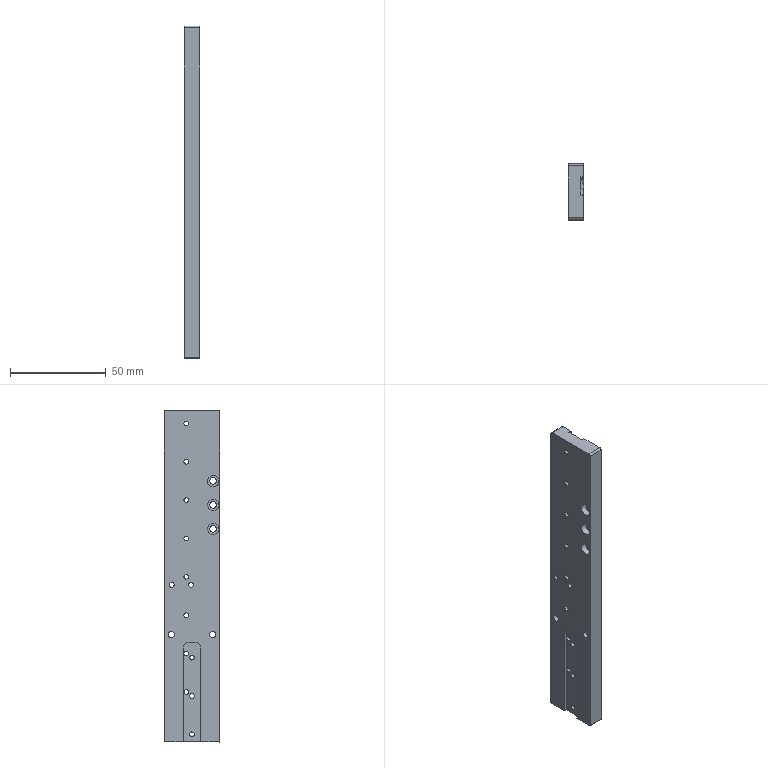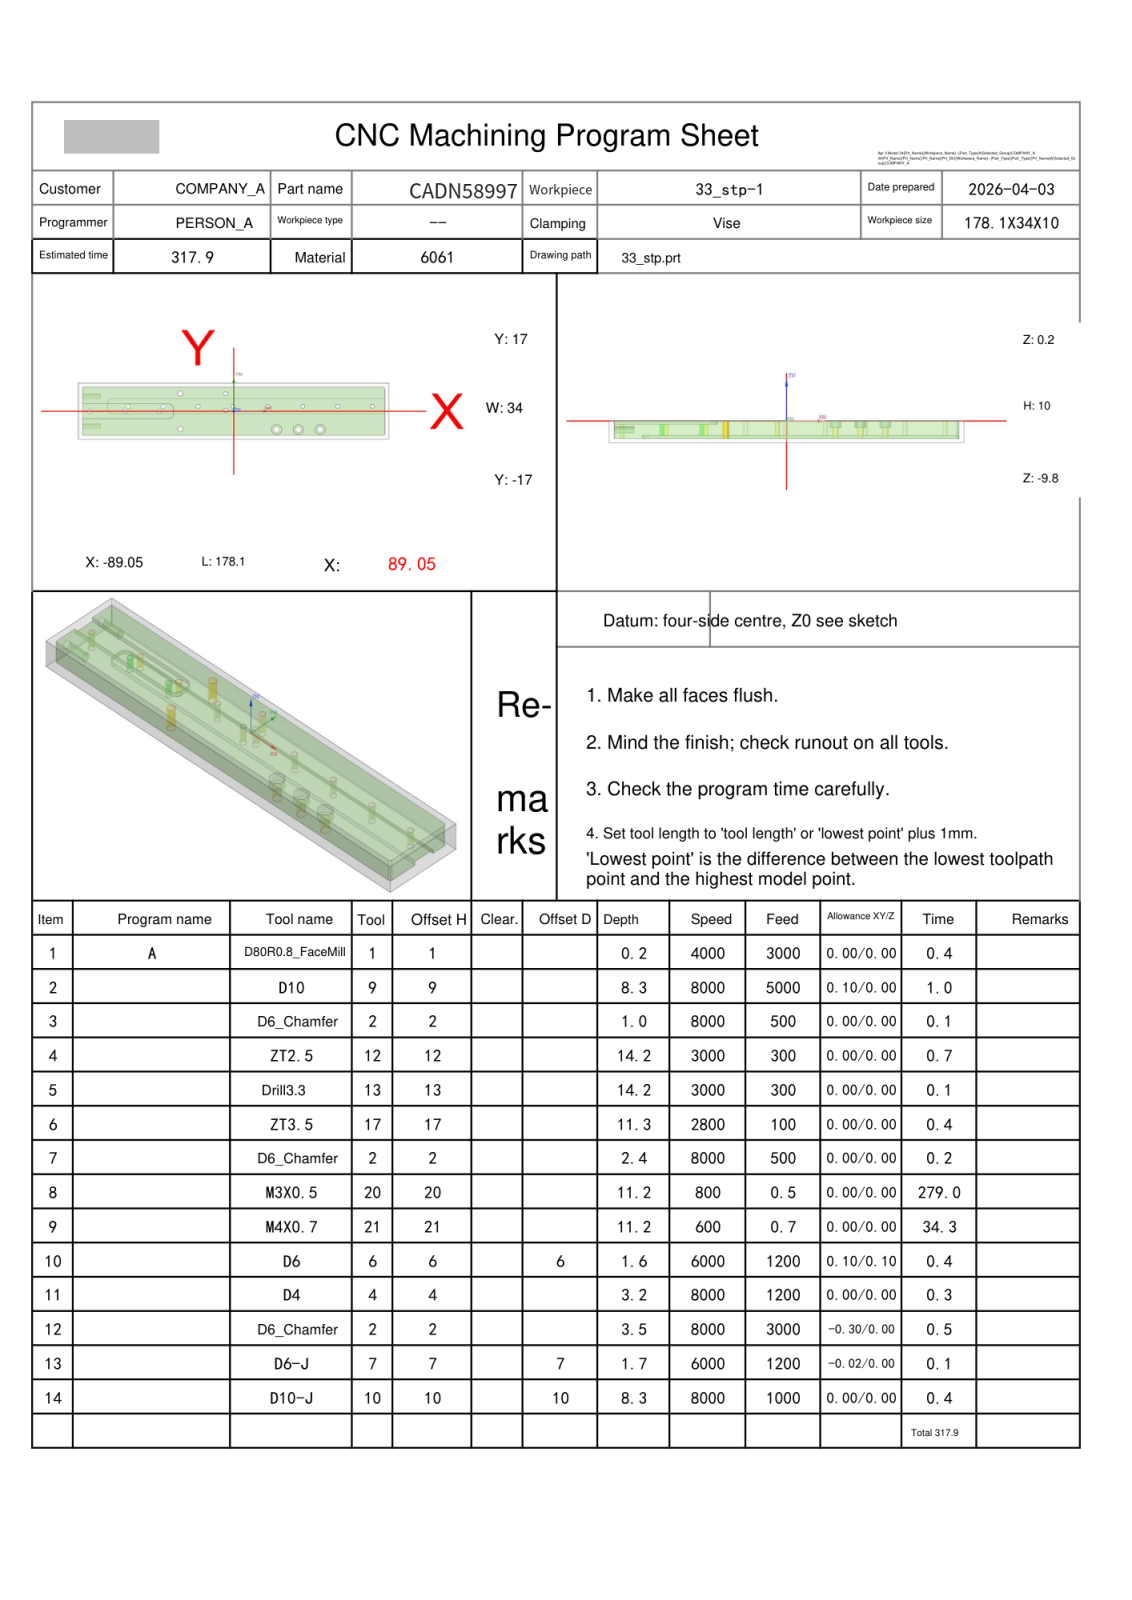NC program | NX | posted by the shop | part box 8 x 29 x 173.1 mm
Whole program:
%
O0001
(Machine time: 605.15 MIN)
(===Total Tool:12===)
(T1=D80R0.8 FaceMill D=80.  R=0.8  D-  H01 Z=-0.   )
(T9=D10     D=10.  R=0.   D-  H09 Z=-8.1  )
(T2=D6 Chamfer   D=6.   R=0.   D-  H02 Z=-3.25 )
(T12=ZT2.5  D=2.5  DR_a=118 D-  H12 Z=-14.  )
(T13=Drill 3.3  D=3.3  DR_a=118 D-  H13 Z=-13.99)
(T17=ZT3.5  D=3.5  DR_a=118 D-  H17 Z=-11.05)
(T20=M3X0.5 D=2.5  DR_a=180 D-  H20 Z=-11.  )
(T21=M4X0.7 D=3.3  DR_a=180 D-  H21 Z=-11.  )
(T6=D6      D=6.   R=0.   D6  H06 Z=-1.4  )
(T4=D4      D=4.   R=0.   D4  H04 Z=-3.   )
(T7=D6-J    D=6.   R=0.   D7  H07 Z=-1.5  )
(T10=D10-J  D=10.  R=0.   D10 H10 Z=-8.1  )
G80 G90 G17 G49 G40
G91 G28 Z0
M01
N1 T01 M06
(D80R0.8 FaceMill  D=80. R=0.8 H=01 ce=0.20 di=0.10)
G00 G90 G54 X-131.55 Y0.0 M03 S4000
G43 H01 Z20.
M08
Z2.1
G01 Z.1 F3000.
X-126.55
X126.55
X131.55
Z2.1
G00 Z20.
G00 G90 X-131.55 Y0.0 M03 S4000
Z20.
Z2.
G01 Z0.0 F1000.
X-126.55
X126.55
X131.55
Z2.
G00 Z20.
G91 G28 Z0.0
M05
M09
G91 G28 Z0.0
M01
N2 T09 M06
(D10  D=10. R=0. H=09 ce=0.10 di=0.00)
G00 G90 G54 X-.4 Y-19.6 M03 S8000
G43 H09 Z20.
M08
Z.5
G01 X-86.35 Z.346 F5000.
G02 X-89.956 Y-18.106 Z.338 I0.0 J5.1
G01 X-90.156 Y-17.906
G02 X-91.65 Y-14.3 Z.331 I3.606 J3.606
G01 Y14.3 Z.279
G02 X-90.156 Y17.906 Z.272 I5.1 J0.0
G01 X-89.956 Y18.106
G02 X-86.35 Y19.6 Z.264 I3.606 J-3.606
G01 X85.55 Z-.044
G02 X91.65 Y13.5 Z-.062 I0.0 J-6.1
G01 Y-13.5 Z-.11
G02 X89.12 Y-18.446 Z-.121 I-6.1 J0.0
X85.55 Y-19.6 Z-.127 I-3.57 J4.946
G01 X-86.35 Z-.436
G02 X-89.956 Y-18.106 Z-.443 I0.0 J5.1
G01 X-90.156 Y-17.906 Z-.444
G02 X-91.65 Y-14.3 Z-.451 I3.606 J3.606
G01 Y14.3 Z-.503
G02 X-90.156 Y17.906 Z-.51 I5.1 J0.0
G01 X-89.956 Y18.106
G02 X-86.35 Y19.6 Z-.517 I3.606 J-3.606
G01 X85.55 Z-.826
G02 X91.65 Y13.5 Z-.843 I0.0 J-6.1
G01 Y-13.5 Z-.892
G02 X89.12 Y-18.446 Z-.902 I-6.1 J0.0
X85.55 Y-19.6 Z-.909 I-3.57 J4.946
G01 X-86.35 Z-1.218
G02 X-89.956 Y-18.106 Z-1.225 I0.0 J5.1
G01 X-90.156 Y-17.906 Z-1.226
G02 X-91.65 Y-14.3 Z-1.233 I3.606 J3.606
G01 Y14.3 Z-1.284
G02 X-90.156 Y17.906 Z-1.292 I5.1 J0.0
G01 X-89.956 Y18.106
G02 X-86.35 Y19.6 Z-1.299 I3.606 J-3.606
G01 X85.55 Z-1.608
G02 X91.65 Y13.5 Z-1.625 I0.0 J-6.1
G01 Y-13.5 Z-1.674
G02 X89.12 Y-18.446 Z-1.684 I-6.1 J0.0
X85.55 Y-19.6 Z-1.691 I-3.57 J4.946
G01 X-86.35 Z-2.
G02 X-89.956 Y-18.106 Z-2.007 I0.0 J5.1
G01 X-90.156 Y-17.906 Z-2.008
G02 X-91.65 Y-14.3 Z-2.015 I3.606 J3.606
G01 Y14.3 Z-2.066
G02 X-90.156 Y17.906 Z-2.073 I5.1 J0.0
G01 X-89.956 Y18.106 Z-2.074
G02 X-86.35 Y19.6 Z-2.081 I3.606 J-3.606
G01 X85.55 Z-2.39
G02 X91.65 Y13.5 Z-2.407 I0.0 J-6.1
G01 Y-13.5 Z-2.456
G02 X89.12 Y-18.446 Z-2.466 I-6.1 J0.0
X85.55 Y-19.6 Z-2.473 I-3.57 J4.946
G01 X-86.35 Z-2.782
G02 X-89.956 Y-18.106 Z-2.789 I0.0 J5.1
G01 X-90.156 Y-17.906
G02 X-91.65 Y-14.3 Z-2.797 I3.606 J3.606
G01 Y14.3 Z-2.848
G02 X-90.156 Y17.906 Z-2.855 I5.1 J0.0
G01 X-89.956 Y18.106 Z-2.856
G02 X-86.35 Y19.6 Z-2.863 I3.606 J-3.606
G01 X85.55 Z-3.172
G02 X91.65 Y13.5 Z-3.189 I0.0 J-6.1
G01 Y-13.5 Z-3.237
G02 X89.12 Y-18.446 Z-3.248 I-6.1 J0.0
X85.55 Y-19.6 Z-3.255 I-3.57 J4.946
G01 X-86.35 Z-3.564
G02 X-89.956 Y-18.106 Z-3.571 I0.0 J5.1
G01 X-90.156 Y-17.906
G02 X-91.65 Y-14.3 Z-3.578 I3.606 J3.606
G01 Y14.3 Z-3.63
G02 X-90.156 Y17.906 Z-3.637 I5.1 J0.0
G01 X-89.956 Y18.106 Z-3.638
G02 X-86.35 Y19.6 Z-3.645 I3.606 J-3.606
G01 X85.55 Z-3.954
G02 X91.65 Y13.5 Z-3.971 I0.0 J-6.1
G01 Y-13.5 Z-4.019
G02 X89.12 Y-18.446 Z-4.03 I-6.1 J0.0
X85.55 Y-19.6 Z-4.036 I-3.57 J4.946
G01 X-86.35 Z-4.345
G02 X-89.956 Y-18.106 Z-4.353 I0.0 J5.1
G01 X-90.156 Y-17.906
G02 X-91.65 Y-14.3 Z-4.36 I3.606 J3.606
G01 Y14.3 Z-4.412
G02 X-90.156 Y17.906 Z-4.419 I5.1 J0.0
G01 X-89.956 Y18.106
G02 X-86.35 Y19.6 Z-4.427 I3.606 J-3.606
G01 X85.55 Z-4.735
G02 X91.65 Y13.5 Z-4.753 I0.0 J-6.1
G01 Y-13.5 Z-4.801
G02 X89.12 Y-18.446 Z-4.811 I-6.1 J0.0
X85.55 Y-19.6 Z-4.818 I-3.57 J4.946
G01 X-86.35 Z-5.127
G02 X-89.956 Y-18.106 Z-5.134 I0.0 J5.1
G01 X-90.156 Y-17.906 Z-5.135
G02 X-91.65 Y-14.3 Z-5.142 I3.606 J3.606
G01 Y14.3 Z-5.193
G02 X-90.156 Y17.906 Z-5.201 I5.1 J0.0
G01 X-89.956 Y18.106
G02 X-86.35 Y19.6 Z-5.208 I3.606 J-3.606
G01 X85.55 Z-5.517
G02 X91.65 Y13.5 Z-5.534 I0.0 J-6.1
G01 Y-13.5 Z-5.583
G02 X89.12 Y-18.446 Z-5.593 I-6.1 J0.0
X85.55 Y-19.6 Z-5.6 I-3.57 J4.946
G01 X-86.35 Z-5.909
G02 X-89.956 Y-18.106 Z-5.916 I0.0 J5.1
G01 X-90.156 Y-17.906 Z-5.917
G02 X-91.65 Y-14.3 Z-5.924 I3.606 J3.606
G01 Y14.3 Z-5.975
G02 X-90.156 Y17.906 Z-5.982 I5.1 J0.0
G01 X-89.956 Y18.106 Z-5.983
G02 X-86.35 Y19.6 Z-5.99 I3.606 J-3.606
G01 X85.55 Z-6.299
G02 X91.65 Y13.5 Z-6.316 I0.0 J-6.1
G01 Y-13.5 Z-6.365
G02 X89.12 Y-18.446 Z-6.375 I-6.1 J0.0
X85.55 Y-19.6 Z-6.382 I-3.57 J4.946
G01 X-86.35 Z-6.691
G02 X-89.956 Y-18.106 Z-6.698 I0.0 J5.1
G01 X-90.156 Y-17.906
G02 X-91.65 Y-14.3 Z-6.706 I3.606 J3.606
G01 Y14.3 Z-6.757
G02 X-90.156 Y17.906 Z-6.764 I5.1 J0.0
G01 X-89.956 Y18.106 Z-6.765
G02 X-86.35 Y19.6 Z-6.772 I3.606 J-3.606
G01 X85.55 Z-7.081
G02 X91.65 Y13.5 Z-7.098 I0.0 J-6.1
G01 Y-13.5 Z-7.147
G02 X89.12 Y-18.446 Z-7.157 I-6.1 J0.0
X85.55 Y-19.6 Z-7.164 I-3.57 J4.946
G01 X-86.35 Z-7.473
G02 X-89.956 Y-18.106 Z-7.48 I0.0 J5.1
G01 X-90.156 Y-17.906
G02 X-91.65 Y-14.3 Z-7.488 I3.606 J3.606
G01 Y14.3 Z-7.539
G02 X-90.156 Y17.906 Z-7.546 I5.1 J0.0
G01 X-89.956 Y18.106 Z-7.547
G02 X-86.35 Y19.6 Z-7.554 I3.606 J-3.606
G01 X85.55 Z-7.863
G02 X91.65 Y13.5 Z-7.88 I0.0 J-6.1
G01 Y-13.5 Z-7.928
G02 X89.12 Y-18.446 Z-7.939 I-6.1 J0.0
X85.55 Y-19.6 Z-7.946 I-3.57 J4.946
G01 X-.4 Z-8.1
X-86.35
G02 X-89.956 Y-18.106 I0.0 J5.1
G01 X-90.156 Y-17.906
G02 X-91.65 Y-14.3 I3.606 J3.606
G01 Y14.3
G02 X-90.156 Y17.906 I5.1 J0.0
G01 X-89.956 Y18.106
G02 X-86.35 Y19.6 I3.606 J-3.606
G01 X85.55
G02 X91.65 Y13.5 I0.0 J-6.1
G01 Y-13.5
G02 X85.55 Y-19.6 I-6.1 J0.0
G01 X-.4
X-.9
Z-7.1
G00 Z20.
G91 G28 Z0.0
M05
M09
G91 G28 Z0.0
M01
N3 T02 M06
(D6 Chamfer  D=6. R=0. H=02 ce=0.00 di=0.00)
G00 G90 G54 X79.55 Y3. M03 S8000
G43 H02 Z20.
M08
G98 G81 X79.55 Y3. Z-.8 R1. F500.
X59.55
X49.55 Y-11.045
X39.55 Y3.
X37.05 Y-11.045
X24.55
X19.55 Y3.
X-.45
X-4.574 Y.55
Y10.55
X-20.45 Y3.
X-30.55 Y-10.75
Y10.75
X-40.45 Y3.
X-42.55 Y0.0
X-60.45 Y3.
X-62.55 Y0.0
X-82.55
G80
G00 Z20.
G91 G28 Z0.0
M05
M09
G91 G28 Z0.0
M01
N4 T12 M06
(ZT2.5 D=2.5 DR_a=118 H=12)
G00 G90 G54 X79.55 Y3. M03 S3000
G43 H12 Z20.
M08
G98 G83 X79.55 Y3. Z-14. R1. F300. Q2.
X59.55
X39.55
X19.55
X-.45
X-4.574 Y.55
Y10.55
X-20.45 Y3.
X-40.45
X-42.55 Y0.0
X-60.45 Y3.
X-62.55 Y0.0
X-82.55
G80
G00 Z20.
G91 G28 Z0.0
M05
M09
G91 G28 Z0.0
M01
N5 T13 M06
(Drill 3.3 D=3.3 DR_a=118 H=13)
G00 G90 G54 X-30.55 Y10.75 M03 S3000
G43 H13 Z20.
M08
G98 G83 X-30.55 Y10.75 Z-13.991 R1. F300. Q2.
Y-10.75
G80
G00 Z20.
G91 G28 Z0.0
M05
M09
G91 G28 Z0.0
M01
N6 T17 M06
(ZT3.5 D=3.5 DR_a=118 H=17)
G00 G90 G54 X49.55 Y-11.045 M03 S2800
G43 H17 Z20.
M08
G98 G83 X49.55 Y-11.045 Z-11.052 R1. F100. Q2.
X37.05
X24.55
G80
G00 Z20.
G91 G28 Z0.0
M05
M09
G91 G28 Z0.0
M01
N7 T02 M06
(D6 Chamfer  D=6. R=0. H=02 ce=0.00 di=0.00)
G00 G90 G54 X79.55 Y3. M03 S8000
G43 H02 Z20.
M08
G98 G81 X79.55 Y3. Z-1.75 R3. F500.
X59.55
X39.55
X19.55
X-.45
X-4.574 Y.55
Y10.55
X-20.45 Y3.
X-40.45
X-42.55 Y0.0
X-60.45 Y3.
X-62.55 Y0.0
X-82.55
G80
G00 Z20.
G00 G90 X-30.55 Y10.75 M03 S8000
Z20.
G98 G81 X-30.55 Y10.75 Z-2.2 R3. F500.
Y-10.75
G80
G00 Z20.
G91 G28 Z0.0
M05
M09
G91 G28 Z0.0
M01
N8 T20 M06
(M3X0.5 D=2.5 DR_a=180 H=20)
G00 G90 G54 X79.55 Y3. M03 S800
G43 H20 Z20.
M08
G95
G98 G84 X79.55 Y3. Z-9.5 R1. F.5 Q5.
X59.55
X39.55
X19.55
X-.45
X-4.574 Y.55
G98 G84 X-4.574 Y10.55 Z-11. R1.
G98 G84 X-20.45 Y3. Z-9.5 R1.
X-40.45
X-42.55 Y0.0
X-60.45 Y3.
X-62.55 Y0.0
G98 G84 X-82.55 Y0.0 Z-11. R1.
G80
G94
G00 Z20.
G91 G28 Z0.0
M05
M09
G91 G28 Z0.0
M01
N9 T21 M06
(M4X0.7 D=3.3 DR_a=180 H=21)
G00 G90 G54 X-30.55 Y10.75 M03 S600
G43 H21 Z20.
M08
G95
G98 G84 X-30.55 Y10.75 Z-11. R1. F.7 Q4.
Y-10.75
G80
G94
G00 Z20.
G91 G28 Z0.0
M05
M09
G91 G28 Z0.0
M01
N10 T06 M06
(D6  D=6. R=0. H=06 ce=0.10 di=0.10)
G00 G90 G54 X-90.25 Y-.335 M03 S6000
G43 H06 Z20.
M08
Z.15
G01 Z-.35 F1200.
G41 D06
Y-.435
G03 X-89.25 Y-1.435 I1. J0.0
G01 X-37.615
Y1.435
X-89.25
G03 X-90.25 Y.435 I0.0 J-1.
G01 G40 Y.335
Z.15
G00 Z20.
Y-.335
Z-.2
G01 Z-.7
G41 D06
Y-.435
G03 X-89.25 Y-1.435 I1. J0.0
G01 X-37.615
Y1.435
X-89.25
G03 X-90.25 Y.435 I0.0 J-1.
G01 G40 Y.335
Z-.2
G00 Z20.
Y-.335
Z-.55
G01 Z-1.05
G41 D06
Y-.435
G03 X-89.25 Y-1.435 I1. J0.0
G01 X-37.615
Y1.435
X-89.25
G03 X-90.25 Y.435 I0.0 J-1.
G01 G40 Y.335
Z-.55
G00 Z20.
Y-.335
Z-.9
G01 Z-1.4
G41 D06
Y-.435
G03 X-89.25 Y-1.435 I1. J0.0
G01 X-37.615
Y1.435
X-89.25
G03 X-90.25 Y.435 I0.0 J-1.
G01 G40 Y.335
Z-.9
G00 Z20.
G91 G28 Z0.0
M05
M09
G91 G28 Z0.0
M01
N11 T04 M06
(D4  D=4. R=0. H=04 ce=0.10 di=0.00)
G00 G90 G54 X49.55 Y-11.045 M03 S8000
G43 H04 Z20.
M08
Z.5
G03 X50. Y-10.595 I0.0 J.45 F1200.
X49.55 Y-10.145 I-.45 J0.0
X49.55 Y-10.145 Z.2 I0.0 J-.9
X49.55 Y-10.145 Z-.1 I0.0 J-.9
X49.55 Y-10.145 Z-.4 I0.0 J-.9
X49.55 Y-10.145 Z-.7 I0.0 J-.9
X49.55 Y-10.145 Z-1. I0.0 J-.9
X49.55 Y-10.145 Z-1.3 I0.0 J-.9
X49.55 Y-10.145 Z-1.6 I0.0 J-.9
X49.55 Y-10.145 Z-1.9 I0.0 J-.9
X49.55 Y-10.145 Z-2.2 I0.0 J-.9
X49.55 Y-10.145 Z-2.5 I0.0 J-.9
X49.55 Y-10.145 Z-2.8 I0.0 J-.9
X50.329 Y-11.495 Z-3. I0.0 J-.9
X50.45 Y-11.045 I-.779 J.45
X49.55 Y-10.145 I-.9 J0.0
X48.65 Y-11.045 I0.0 J-.9
X49.55 Y-11.945 I.9 J0.0
X50.329 Y-11.495 I0.0 J.9
X50.39 Y-11.27 I-.39 J.225
X49.94 Y-10.82 I-.45 J0.0
X49.55 Y-11.045 I0.0 J-.45
G00 Z20.
X37.05
Z.5
G03 X37.5 Y-10.595 I0.0 J.45
X37.05 Y-10.145 I-.45 J0.0
X37.05 Y-10.145 Z.2 I0.0 J-.9
X37.05 Y-10.145 Z-.1 I0.0 J-.9
X37.05 Y-10.145 Z-.4 I0.0 J-.9
X37.05 Y-10.145 Z-.7 I0.0 J-.9
X37.05 Y-10.145 Z-1. I0.0 J-.9
X37.05 Y-10.145 Z-1.3 I0.0 J-.9
X37.05 Y-10.145 Z-1.6 I0.0 J-.9
X37.05 Y-10.145 Z-1.9 I0.0 J-.9
X37.05 Y-10.145 Z-2.2 I0.0 J-.9
X37.05 Y-10.145 Z-2.5 I0.0 J-.9
X37.05 Y-10.145 Z-2.8 I0.0 J-.9
X37.829 Y-11.495 Z-3. I0.0 J-.9
X37.95 Y-11.045 I-.779 J.45
X37.05 Y-10.145 I-.9 J0.0
X36.15 Y-11.045 I0.0 J-.9
X37.05 Y-11.945 I.9 J0.0
X37.829 Y-11.495 I0.0 J.9
X37.89 Y-11.27 I-.39 J.225
X37.44 Y-10.82 I-.45 J0.0
X37.05 Y-11.045 I0.0 J-.45
G00 Z20.
X24.55
Z.5
G03 X25. Y-10.595 I0.0 J.45
X24.55 Y-10.145 I-.45 J0.0
X24.55 Y-10.145 Z.2 I0.0 J-.9
X24.55 Y-10.145 Z-.1 I0.0 J-.9
X24.55 Y-10.145 Z-.4 I0.0 J-.9
X24.55 Y-10.145 Z-.7 I0.0 J-.9
X24.55 Y-10.145 Z-1. I0.0 J-.9
X24.55 Y-10.145 Z-1.3 I0.0 J-.9
X24.55 Y-10.145 Z-1.6 I0.0 J-.9
X24.55 Y-10.145 Z-1.9 I0.0 J-.9
X24.55 Y-10.145 Z-2.2 I0.0 J-.9
X24.55 Y-10.145 Z-2.5 I0.0 J-.9
X24.55 Y-10.145 Z-2.8 I0.0 J-.9
X25.329 Y-11.495 Z-3. I0.0 J-.9
X25.45 Y-11.045 I-.779 J.45
X24.55 Y-10.145 I-.9 J0.0
X23.65 Y-11.045 I0.0 J-.9
X24.55 Y-11.945 I.9 J0.0
X25.329 Y-11.495 I0.0 J.9
X25.39 Y-11.27 I-.39 J.225
X24.94 Y-10.82 I-.45 J0.0
X24.55 Y-11.045 I0.0 J-.45
G00 Z20.
G00 G90 X49.55 Y-11.045 M03 S8000
Z20.
Z.5
G41 D04
G01 X49.735 Y-10.968 F500.
G03 X50.03 Y-10.525 I-.185 J.443
X49.55 Y-10.045 I-.48 J0.0
X50.501 Y-11.354 Z-3. I0.0 J-1.
X50.55 Y-11.045 I-.951 J.309
X49.55 Y-10.045 I-1. J0.0
X48.55 Y-11.045 I0.0 J-1.
X49.55 Y-12.045 I1. J0.0
X50.501 Y-11.354 I0.0 J1.
G01 X50.525 Y-11.206
G03 X50.045 Y-10.726 I-.48 J0.0
X49.68 Y-10.893 I0.0 J-.48
G01 G40 X49.55 Y-11.045
G00 Z20.
X37.05
Z.5
G41 D04
G01 X37.235 Y-10.968
G03 X37.53 Y-10.525 I-.185 J.443
X37.05 Y-10.045 I-.48 J0.0
X38.001 Y-11.354 Z-3. I0.0 J-1.
X38.05 Y-11.045 I-.951 J.309
X37.05 Y-10.045 I-1. J0.0
X36.05 Y-11.045 I0.0 J-1.
X37.05 Y-12.045 I1. J0.0
X38.001 Y-11.354 I0.0 J1.
G01 X38.025 Y-11.206
G03 X37.545 Y-10.726 I-.48 J0.0
X37.18 Y-10.893 I0.0 J-.48
G01 G40 X37.05 Y-11.045
G00 Z20.
X24.55
Z.5
G41 D04
G01 X24.735 Y-10.968
G03 X25.03 Y-10.525 I-.185 J.443
X24.55 Y-10.045 I-.48 J0.0
X25.501 Y-11.354 Z-3. I0.0 J-1.
X25.55 Y-11.045 I-.951 J.309
X24.55 Y-10.045 I-1. J0.0
X23.55 Y-11.045 I0.0 J-1.
X24.55 Y-12.045 I1. J0.0
X25.501 Y-11.354 I0.0 J1.
G01 X25.525 Y-11.206
G03 X25.045 Y-10.726 I-.48 J0.0
X24.68 Y-10.893 I0.0 J-.48
G01 G40 X24.55 Y-11.045
G00 Z20.
G91 G28 Z0.0
M05
M09
G91 G28 Z0.0
M01
N12 T02 M06
(D6 Chamfer  D=6. R=0. H=02 ce=0.00 di=0.00)
G00 G90 G54 X-82.55 Y0.0 M03 S8000
G43 H02 Z20.
M08
G98 G81 X-82.55 Y0.0 Z-3.25 R1.5 F500.
X-62.55
X-42.55
X-20.45 Y3. Z-1.75 R3.
X-4.574 Y.55
X-.45 Y3.
X-4.574 Y10.55
X19.55 Y3.
X39.55
X59.55
X79.55
G80
G00 Z20.
G00 G90 X-.15 Y-16.628 M03 S8000
Z20.
Z2.099
G01 Z-1.5 F3000.
G03 X-.07 Y-16.328 I-.52 J.3
X-.37 Y-15.808 I-.6 J0.0
G01 X-.4 Y-15.8
X-86.35
X-86.604 Y-15.775
X-86.847 Y-15.701
X-87.072 Y-15.581
X-87.269 Y-15.419
X-87.469 Y-15.219
X-87.631 Y-15.022
X-87.751 Y-14.797
X-87.825 Y-14.554
X-87.85 Y-14.3
Y-4.535
G02 X-86.55 Y-3.235 I1.3 J0.0
G01 X-37.55
G03 X-35.815 Y-1.5 I0.0 J1.735
G01 Y1.5
G03 X-37.55 Y3.235 I-1.735 J0.0
G01 X-86.55
G02 X-87.85 Y4.535 I0.0 J1.3
G01 Y14.3
X-87.825 Y14.554
X-87.751 Y14.797
X-87.631 Y15.022
X-87.469 Y15.219
X-87.269 Y15.419
X-87.072 Y15.581
X-86.847 Y15.701
X-86.604 Y15.775
X-86.35 Y15.8
X85.55
G02 X87.85 Y13.5 I0.0 J-2.3
G01 Y-13.5
G02 X85.55 Y-15.8 I-2.3 J0.0
G01 X-.4
X-.43 Y-15.808
G03 X-.73 Y-16.328 I.3 J-.52
X-.65 Y-16.628 I.6 J0.0
G01 Z2.099
G00 Z20.
X-87.85 Y-1.842
Z1.755
G01 Z-3.
Y1.842
Z1.755
G00 Z20.
G00 G90 X50.72 Y-13.026 M03 S8000
Z20.
Z2.5
G01 X50.802 Y-12.978 Z2.465 F500.
X51.063 Y-12.781 Z2.346
X51.294 Y-12.549 Z2.227
X51.49 Y-12.286 Z2.108
X51.646 Y-11.999 Z1.989
X51.76 Y-11.692 Z1.87
X51.83 Y-11.372 Z1.75
X51.853 Y-11.045 Z1.631
X51.83 Y-10.718 Z1.512
X51.76 Y-10.398 Z1.393
X51.646 Y-10.091 Z1.274
X51.49 Y-9.804 Z1.154
X51.294 Y-9.541 Z1.035
X51.063 Y-9.309 Z.916
X50.802 Y-9.112 Z.797
X50.598 Y-8.994 Z.711
X50.297 Y-8.866 Z.592
X49.98 Y-8.783 Z.473
X49.655 Y-8.744 Z.354
X49.328 Y-8.753 Z.235
X49.005 Y-8.807 Z.115
X48.693 Y-8.907 Z-.004
X48.399 Y-9.051 Z-.123
X48.127 Y-9.234 Z-.242
X47.885 Y-9.454 Z-.361
X47.676 Y-9.706 Z-.48
X47.505 Y-9.986 Z-.6
X47.376 Y-10.286 Z-.719
X47.29 Y-10.602 Z-.838
X47.25 Y-10.927 Z-.957
Y-11.045 Z-1.
G03 X49.55 Y-13.345 I2.3 J0.0
X51.85 Y-11.045 I0.0 J2.3
X49.55 Y-8.745 I-2.3 J0.0
X47.25 Y-11.045 I0.0 J-2.3
X47.304 Y-11.541 I2.3 J0.0
G01 Z1.5
G00 Z20.
X38.22 Y-13.026
Z2.5
G01 X38.302 Y-12.978 Z2.465
X38.563 Y-12.781 Z2.346
X38.794 Y-12.549 Z2.227
X38.99 Y-12.286 Z2.108
X39.146 Y-11.999 Z1.989
X39.26 Y-11.692 Z1.87
X39.33 Y-11.372 Z1.75
X39.353 Y-11.045 Z1.631
X39.33 Y-10.718 Z1.512
X39.26 Y-10.398 Z1.393
X39.146 Y-10.091 Z1.274
X38.99 Y-9.804 Z1.154
X38.794 Y-9.541 Z1.035
X38.563 Y-9.309 Z.916
X38.302 Y-9.112 Z.797
X38.098 Y-8.994 Z.711
X37.797 Y-8.866 Z.592
X37.48 Y-8.783 Z.473
X37.155 Y-8.744 Z.354
X36.828 Y-8.753 Z.235
X36.505 Y-8.807 Z.115
X36.193 Y-8.907 Z-.004
X35.899 Y-9.051 Z-.123
X35.627 Y-9.234 Z-.242
X35.385 Y-9.454 Z-.361
X35.176 Y-9.706 Z-.48
X35.005 Y-9.986 Z-.6
X34.876 Y-10.286 Z-.719
X34.79 Y-10.602 Z-.838
X34.75 Y-10.927 Z-.957
Y-11.045 Z-1.
G03 X37.05 Y-13.345 I2.3 J0.0
X39.35 Y-11.045 I0.0 J2.3
X37.05 Y-8.745 I-2.3 J0.0
X34.75 Y-11.045 I0.0 J-2.3
X34.804 Y-11.541 I2.3 J0.0
G01 Z1.5
G00 Z20.
X25.72 Y-13.026
Z2.5
G01 X25.802 Y-12.978 Z2.465
X26.063 Y-12.781 Z2.346
X26.294 Y-12.549 Z2.227
X26.49 Y-12.286 Z2.108
X26.646 Y-11.999 Z1.989
X26.76 Y-11.692 Z1.87
X26.83 Y-11.372 Z1.75
X26.853 Y-11.045 Z1.631
X26.83 Y-10.718 Z1.512
X26.76 Y-10.398 Z1.393
X26.646 Y-10.091 Z1.274
X26.49 Y-9.804 Z1.154
X26.294 Y-9.541 Z1.035
X26.063 Y-9.309 Z.916
X25.802 Y-9.112 Z.797
X25.598 Y-8.994 Z.711
X25.297 Y-8.866 Z.592
X24.98 Y-8.783 Z.473
X24.655 Y-8.744 Z.354
X24.328 Y-8.753 Z.235
X24.005 Y-8.807 Z.115
X23.693 Y-8.907 Z-.004
X23.399 Y-9.051 Z-.123
X23.127 Y-9.234 Z-.242
X22.885 Y-9.454 Z-.361
X22.676 Y-9.706 Z-.48
X22.505 Y-9.986 Z-.6
X22.376 Y-10.286 Z-.719
X22.29 Y-10.602 Z-.838
X22.25 Y-10.927 Z-.957
Y-11.045 Z-1.
G03 X24.55 Y-13.345 I2.3 J0.0
X26.85 Y-11.045 I0.0 J2.3
X24.55 Y-8.745 I-2.3 J0.0
X22.25 Y-11.045 I0.0 J-2.3
X22.304 Y-11.541 I2.3 J0.0
G01 Z1.5
G00 Z20.
G91 G28 Z0.0
M05
M09
G91 G28 Z0.0
M01
N13 T07 M06
(D6-J  D=6. R=0. H=07 ce=-0.02 di=0.00)
G00 G90 G54 X-90.25 Y-.455 M03 S6000
G43 H07 Z20.
M08
Z-1.
G01 Z-1.5 F1200.
G41 D07
Y-.555
G03 X-89.25 Y-1.555 I1. J0.0
G01 X-37.55
X-37.518 Y-1.556
X-37.494 Y-1.533
X-37.495 Y-1.5
Y1.5
X-37.494 Y1.533
X-37.518 Y1.556
X-37.55 Y1.555
X-89.25
G03 X-90.25 Y.555 I0.0 J-1.
G01 G40 Y.455
Z-1.
G00 Z20.
G91 G28 Z0.0
M05
M09
G91 G28 Z0.0
M01
N14 T10 M06
(D10-J  D=10. R=0. H=10 ce=0.00 di=0.00)
G00 G90 G54 X-87.363 Y20.616 M03 S8000
G43 H10 Z20.
M08
Z-7.6
G01 Z-8.1 F1000.
G41 D10
X-87.347 Y20.417
G03 X-86.35 Y19.5 I.997 J.083
G01 X85.55
G02 X91.55 Y13.5 I0.0 J-6.
G01 Y7.735
Y-13.5
G02 X85.55 Y-19.5 I-6. J0.0
G01 X-86.35
G02 X-89.886 Y-18.036 I0.0 J5.
G01 X-90.086 Y-17.836
G02 X-91.55 Y-14.3 I3.536 J3.536
G01 Y14.3
G02 X-90.086 Y17.836 I5. J0.0
G01 X-89.886 Y18.036
G02 X-86.35 Y19.5 I3.536 J-3.536
G01 X-85.85
G03 X-84.85 Y20.5 I0.0 J1.
G01 G40 Y20.7
Z-7.6
G00 Z20.
M05
M09
G91 G28 Z0.0
G91 G28 Y0.0
M30
%